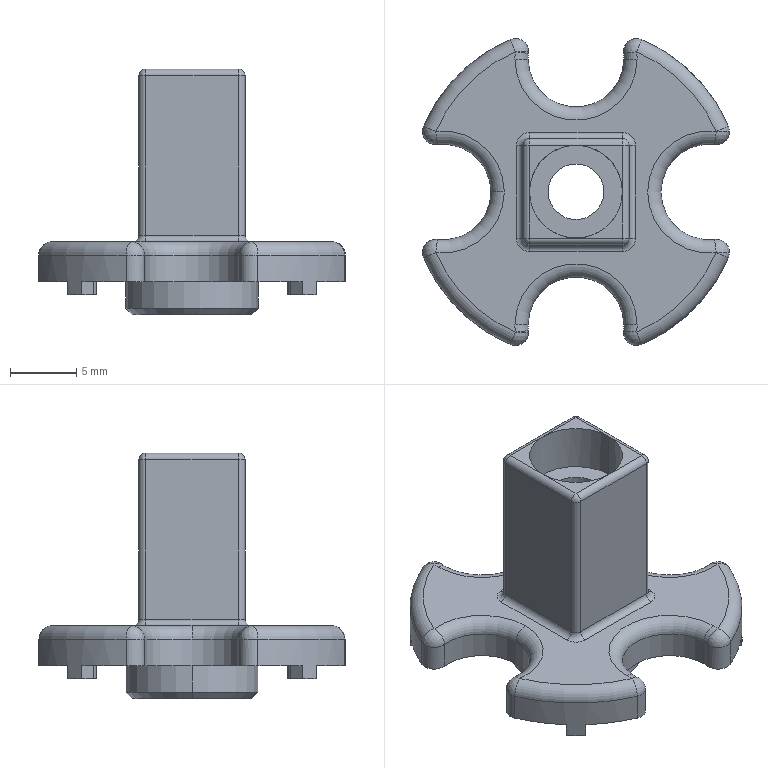Part | SolidWorks | features ICE 6, Fillet 3, Chamfer 1, Extrusion 1, RevCut 1 | 1 solid | 127 faces | box 23.109 x 23.109 x 18.5 mm | volume 1457 mm3 | cylinder 53 | plane 33 | sphere 18 | torus 17 | cone 6 | commonest cylinder face diameters 1 x12 2 x12 7.2 x9 1.5 x6 6.5 x4 25 x4